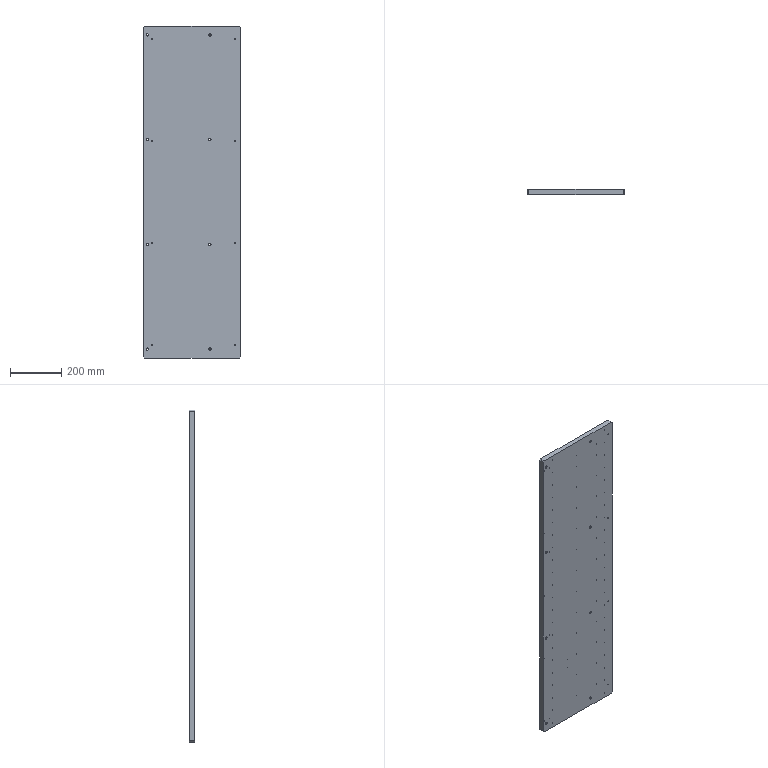Part | NX | features BREP 1 | 1 solid | 446 faces | box 380 x 20 x 1300 mm | volume 9827931 mm3 | cylinder 242 | cone 178 | plane 26 | commonest cylinder face diameters 5 x158 9 x32 3.3 x24 15 x16 6 x12